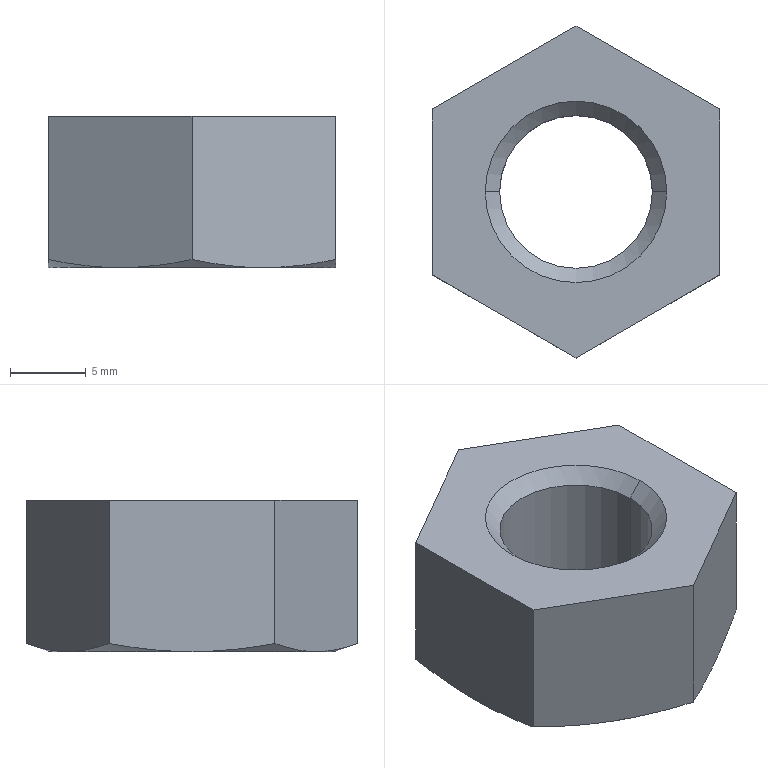Part | SolidWorks | features BaseBody 1 | 1 solid | 20 faces | box 19 x 21.939 x 10 mm | volume 2289 mm3 | cone 10 | plane 8 | cylinder 2 | commonest cylinder face diameters 10.106 x2
STEP:
#1=CARTESIAN_POINT('',(-5.053,0.,0.947));
#2=VERTEX_POINT('',#1);
#3=CARTESIAN_POINT('',(5.053,0.,0.947));
#4=VERTEX_POINT('',#3);
#5=CARTESIAN_POINT('',(0.,0.,0.947));
#6=DIRECTION('',(0.,0.,1.));
#7=DIRECTION('',(1.,0.,0.));
#8=AXIS2_PLACEMENT_3D('',#5,#6,#7);
#9=CIRCLE('',#8,5.053);
#10=EDGE_CURVE('',#2,#4,#9,.T.);
#11=ORIENTED_EDGE('',*,*,#10,.F.);
#12=CARTESIAN_POINT('',(-5.053,0.,9.053));
#13=VERTEX_POINT('',#12);
#14=CARTESIAN_POINT('',(-5.053,0.,0.));
#15=DIRECTION('',(0.,0.,1.));
#16=VECTOR('',#15,1000.);
#17=LINE('',#14,#16);
#18=EDGE_CURVE('',#2,#13,#17,.T.);
#19=ORIENTED_EDGE('',*,*,#18,.T.);
#20=CARTESIAN_POINT('',(5.053,0.,9.053));
#21=VERTEX_POINT('',#20);
#22=CARTESIAN_POINT('',(0.,0.,9.053));
#23=DIRECTION('',(0.,0.,-1.));
#24=DIRECTION('',(1.,0.,0.));
#25=AXIS2_PLACEMENT_3D('',#22,#23,#24);
#26=CIRCLE('',#25,5.053);
#27=EDGE_CURVE('',#21,#13,#26,.T.);
#28=ORIENTED_EDGE('',*,*,#27,.F.);
#29=CARTESIAN_POINT('',(5.053,0.,0.));
#30=DIRECTION('',(0.,0.,1.));
#31=VECTOR('',#30,1000.);
#32=LINE('',#29,#31);
#33=EDGE_CURVE('',#4,#21,#32,.T.);
#34=ORIENTED_EDGE('',*,*,#33,.F.);
#35=EDGE_LOOP('',(#11,#19,#28,#34));
#36=FACE_OUTER_BOUND('',#35,.T.);
#37=CARTESIAN_POINT('',(0.,0.,0.));
#38=DIRECTION('',(0.,0.,1.));
#39=DIRECTION('',(1.,0.,0.));
#40=AXIS2_PLACEMENT_3D('',#37,#38,#39);
#41=CYLINDRICAL_SURFACE('',#40,5.053);
#42=ADVANCED_FACE('',(#36),#41,.F.);
#43=ORIENTED_EDGE('',*,*,#27,.T.);
#44=CARTESIAN_POINT('',(-6.,0.,10.));
#45=VERTEX_POINT('',#44);
#46=CARTESIAN_POINT('',(-6.,0.,10.));
#47=DIRECTION('',(-0.7071,0.,0.7071));
#48=VECTOR('',#47,1000.);
#49=LINE('',#46,#48);
#50=EDGE_CURVE('',#13,#45,#49,.T.);
#51=ORIENTED_EDGE('',*,*,#50,.T.);
#52=CARTESIAN_POINT('',(6.,0.,10.));
#53=VERTEX_POINT('',#52);
#54=CARTESIAN_POINT('',(0.,0.,10.));
#55=DIRECTION('',(0.,0.,-1.));
#56=DIRECTION('',(1.,0.,0.));
#57=AXIS2_PLACEMENT_3D('',#54,#55,#56);
#58=CIRCLE('',#57,6.);
#59=EDGE_CURVE('',#53,#45,#58,.T.);
#60=ORIENTED_EDGE('',*,*,#59,.F.);
#61=CARTESIAN_POINT('',(6.,0.,10.));
#62=DIRECTION('',(0.7071,0.,0.7071));
#63=VECTOR('',#62,1000.);
#64=LINE('',#61,#63);
#65=EDGE_CURVE('',#21,#53,#64,.T.);
#66=ORIENTED_EDGE('',*,*,#65,.F.);
#67=EDGE_LOOP('',(#43,#51,#60,#66));
#68=FACE_OUTER_BOUND('',#67,.T.);
#69=CARTESIAN_POINT('',(0.,0.,10.));
#70=DIRECTION('',(0.,0.,1.));
#71=DIRECTION('',(1.,0.,0.));
#72=AXIS2_PLACEMENT_3D('',#69,#70,#71);
#73=CONICAL_SURFACE('',#72,6.,0.7854);
#74=ADVANCED_FACE('',(#68),#73,.F.);
#75=ORIENTED_EDGE('',*,*,#10,.T.);
#76=CARTESIAN_POINT('',(6.,0.,0.));
#77=VERTEX_POINT('',#76);
#78=CARTESIAN_POINT('',(6.,0.,0.));
#79=DIRECTION('',(0.7071,0.,-0.7071));
#80=VECTOR('',#79,1000.);
#81=LINE('',#78,#80);
#82=EDGE_CURVE('',#4,#77,#81,.T.);
#83=ORIENTED_EDGE('',*,*,#82,.T.);
#84=CARTESIAN_POINT('',(-6.,0.,0.));
#85=VERTEX_POINT('',#84);
#86=CARTESIAN_POINT('',(0.,0.,0.));
#87=DIRECTION('',(0.,0.,1.));
#88=DIRECTION('',(-1.,0.,0.));
#89=AXIS2_PLACEMENT_3D('',#86,#87,#88);
#90=CIRCLE('',#89,6.);
#91=EDGE_CURVE('',#85,#77,#90,.T.);
#92=ORIENTED_EDGE('',*,*,#91,.F.);
#93=CARTESIAN_POINT('',(-6.,0.,0.));
#94=DIRECTION('',(-0.7071,0.,-0.7071));
#95=VECTOR('',#94,1000.);
#96=LINE('',#93,#95);
#97=EDGE_CURVE('',#2,#85,#96,.T.);
#98=ORIENTED_EDGE('',*,*,#97,.F.);
#99=EDGE_LOOP('',(#75,#83,#92,#98));
#100=FACE_OUTER_BOUND('',#99,.T.);
#101=CARTESIAN_POINT('',(0.,0.,0.));
#102=DIRECTION('',(0.,0.,-1.));
#103=DIRECTION('',(-1.,0.,0.));
#104=AXIS2_PLACEMENT_3D('',#101,#102,#103);
#105=CONICAL_SURFACE('',#104,6.,0.7854);
#106=ADVANCED_FACE('',(#100),#105,.F.);
#107=ORIENTED_EDGE('',*,*,#18,.F.);
#108=CARTESIAN_POINT('',(0.,0.,0.947));
#109=DIRECTION('',(0.,0.,1.));
#110=DIRECTION('',(1.,0.,0.));
#111=AXIS2_PLACEMENT_3D('',#108,#109,#110);
#112=CIRCLE('',#111,5.053);
#113=EDGE_CURVE('',#4,#2,#112,.T.);
#114=ORIENTED_EDGE('',*,*,#113,.F.);
#115=ORIENTED_EDGE('',*,*,#33,.T.);
#116=CARTESIAN_POINT('',(0.,0.,9.053));
#117=DIRECTION('',(0.,0.,-1.));
#118=DIRECTION('',(1.,0.,0.));
#119=AXIS2_PLACEMENT_3D('',#116,#117,#118);
#120=CIRCLE('',#119,5.053);
#121=EDGE_CURVE('',#13,#21,#120,.T.);
#122=ORIENTED_EDGE('',*,*,#121,.F.);
#123=EDGE_LOOP('',(#107,#114,#115,#122));
#124=FACE_OUTER_BOUND('',#123,.T.);
#125=CARTESIAN_POINT('',(0.,0.,0.));
#126=DIRECTION('',(0.,0.,1.));
#127=DIRECTION('',(1.,0.,0.));
#128=AXIS2_PLACEMENT_3D('',#125,#126,#127);
#129=CYLINDRICAL_SURFACE('',#128,5.053);
#130=ADVANCED_FACE('',(#124),#129,.F.);
#131=ORIENTED_EDGE('',*,*,#50,.F.);
#132=ORIENTED_EDGE('',*,*,#121,.T.);
#133=ORIENTED_EDGE('',*,*,#65,.T.);
#134=CARTESIAN_POINT('',(0.,0.,10.));
#135=DIRECTION('',(0.,0.,-1.));
#136=DIRECTION('',(1.,0.,0.));
#137=AXIS2_PLACEMENT_3D('',#134,#135,#136);
#138=CIRCLE('',#137,6.);
#139=EDGE_CURVE('',#45,#53,#138,.T.);
#140=ORIENTED_EDGE('',*,*,#139,.F.);
#141=EDGE_LOOP('',(#131,#132,#133,#140));
#142=FACE_OUTER_BOUND('',#141,.T.);
#143=CARTESIAN_POINT('',(0.,0.,10.));
#144=DIRECTION('',(0.,0.,1.));
#145=DIRECTION('',(1.,0.,0.));
#146=AXIS2_PLACEMENT_3D('',#143,#144,#145);
#147=CONICAL_SURFACE('',#146,6.,0.7854);
#148=ADVANCED_FACE('',(#142),#147,.F.);
#149=ORIENTED_EDGE('',*,*,#82,.F.);
#150=ORIENTED_EDGE('',*,*,#113,.T.);
#151=ORIENTED_EDGE('',*,*,#97,.T.);
#152=CARTESIAN_POINT('',(0.,0.,0.));
#153=DIRECTION('',(0.,0.,1.));
#154=DIRECTION('',(-1.,0.,0.));
#155=AXIS2_PLACEMENT_3D('',#152,#153,#154);
#156=CIRCLE('',#155,6.);
#157=EDGE_CURVE('',#77,#85,#156,.T.);
#158=ORIENTED_EDGE('',*,*,#157,.F.);
#159=EDGE_LOOP('',(#149,#150,#151,#158));
#160=FACE_OUTER_BOUND('',#159,.T.);
#161=CARTESIAN_POINT('',(0.,0.,0.));
#162=DIRECTION('',(0.,0.,-1.));
#163=DIRECTION('',(-1.,0.,0.));
#164=AXIS2_PLACEMENT_3D('',#161,#162,#163);
#165=CONICAL_SURFACE('',#164,6.,0.7854);
#166=ADVANCED_FACE('',(#160),#165,.F.);
#167=ORIENTED_EDGE('',*,*,#59,.T.);
#168=ORIENTED_EDGE('',*,*,#139,.T.);
#169=EDGE_LOOP('',(#167,#168));
#170=FACE_BOUND('',#169,.T.);
#171=CARTESIAN_POINT('',(9.5,-5.485,10.));
#172=VERTEX_POINT('',#171);
#173=CARTESIAN_POINT('',(9.5,5.485,10.));
#174=VERTEX_POINT('',#173);
#175=CARTESIAN_POINT('',(9.5,0.,10.));
#176=DIRECTION('',(0.,1.,0.));
#177=VECTOR('',#176,1000.);
#178=LINE('',#175,#177);
#179=EDGE_CURVE('',#172,#174,#178,.T.);
#180=ORIENTED_EDGE('',*,*,#179,.T.);
#181=CARTESIAN_POINT('',(0.,10.97,10.));
#182=VERTEX_POINT('',#181);
#183=CARTESIAN_POINT('',(9.5,5.485,10.));
#184=DIRECTION('',(-0.866,0.5,0.));
#185=VECTOR('',#184,1000.);
#186=LINE('',#183,#185);
#187=EDGE_CURVE('',#174,#182,#186,.T.);
#188=ORIENTED_EDGE('',*,*,#187,.T.);
#189=CARTESIAN_POINT('',(-9.5,5.485,10.));
#190=VERTEX_POINT('',#189);
#191=CARTESIAN_POINT('',(0.,10.97,10.));
#192=DIRECTION('',(-0.866,-0.5,0.));
#193=VECTOR('',#192,1000.);
#194=LINE('',#191,#193);
#195=EDGE_CURVE('',#182,#190,#194,.T.);
#196=ORIENTED_EDGE('',*,*,#195,.T.);
#197=CARTESIAN_POINT('',(-9.5,-5.485,10.));
#198=VERTEX_POINT('',#197);
#199=CARTESIAN_POINT('',(-9.5,0.,10.));
#200=DIRECTION('',(0.,-1.,0.));
#201=VECTOR('',#200,1000.);
#202=LINE('',#199,#201);
#203=EDGE_CURVE('',#190,#198,#202,.T.);
#204=ORIENTED_EDGE('',*,*,#203,.T.);
#205=CARTESIAN_POINT('',(0.,-10.97,10.));
#206=VERTEX_POINT('',#205);
#207=CARTESIAN_POINT('',(-9.5,-5.485,10.));
#208=DIRECTION('',(0.866,-0.5,0.));
#209=VECTOR('',#208,1000.);
#210=LINE('',#207,#209);
#211=EDGE_CURVE('',#198,#206,#210,.T.);
#212=ORIENTED_EDGE('',*,*,#211,.T.);
#213=CARTESIAN_POINT('',(0.,-10.97,10.));
#214=DIRECTION('',(0.866,0.5,0.));
#215=VECTOR('',#214,1000.);
#216=LINE('',#213,#215);
#217=EDGE_CURVE('',#206,#172,#216,.T.);
#218=ORIENTED_EDGE('',*,*,#217,.T.);
#219=EDGE_LOOP('',(#180,#188,#196,#204,#212,#218));
#220=FACE_OUTER_BOUND('',#219,.T.);
#221=CARTESIAN_POINT('',(0.,0.,10.));
#222=DIRECTION('',(0.,0.,1.));
#223=DIRECTION('',(1.,0.,0.));
#224=AXIS2_PLACEMENT_3D('',#221,#222,#223);
#225=PLANE('',#224);
#226=ADVANCED_FACE('',(#170,#220),#225,.T.);
#227=ORIENTED_EDGE('',*,*,#91,.T.);
#228=ORIENTED_EDGE('',*,*,#157,.T.);
#229=EDGE_LOOP('',(#227,#228));
#230=FACE_BOUND('',#229,.T.);
#231=CARTESIAN_POINT('',(-4.75,-8.227,0.));
#232=VERTEX_POINT('',#231);
#233=CARTESIAN_POINT('',(4.75,-8.227,0.));
#234=VERTEX_POINT('',#233);
#235=CARTESIAN_POINT('',(0.,0.,0.));
#236=DIRECTION('',(0.,0.,1.));
#237=DIRECTION('',(1.,0.,0.));
#238=AXIS2_PLACEMENT_3D('',#235,#236,#237);
#239=CIRCLE('',#238,9.5);
#240=EDGE_CURVE('',#232,#234,#239,.T.);
#241=ORIENTED_EDGE('',*,*,#240,.F.);
#242=CARTESIAN_POINT('',(-9.5,0.,0.));
#243=VERTEX_POINT('',#242);
#244=CARTESIAN_POINT('',(0.,0.,0.));
#245=DIRECTION('',(0.,0.,1.));
#246=DIRECTION('',(1.,0.,0.));
#247=AXIS2_PLACEMENT_3D('',#244,#245,#246);
#248=CIRCLE('',#247,9.5);
#249=EDGE_CURVE('',#243,#232,#248,.T.);
#250=ORIENTED_EDGE('',*,*,#249,.F.);
#251=CARTESIAN_POINT('',(-4.75,8.227,0.));
#252=VERTEX_POINT('',#251);
#253=CARTESIAN_POINT('',(0.,0.,0.));
#254=DIRECTION('',(0.,0.,1.));
#255=DIRECTION('',(1.,0.,0.));
#256=AXIS2_PLACEMENT_3D('',#253,#254,#255);
#257=CIRCLE('',#256,9.5);
#258=EDGE_CURVE('',#252,#243,#257,.T.);
#259=ORIENTED_EDGE('',*,*,#258,.F.);
#260=CARTESIAN_POINT('',(4.75,8.227,0.));
#261=VERTEX_POINT('',#260);
#262=CARTESIAN_POINT('',(0.,0.,0.));
#263=DIRECTION('',(0.,0.,1.));
#264=DIRECTION('',(1.,0.,0.));
#265=AXIS2_PLACEMENT_3D('',#262,#263,#264);
#266=CIRCLE('',#265,9.5);
#267=EDGE_CURVE('',#261,#252,#266,.T.);
#268=ORIENTED_EDGE('',*,*,#267,.F.);
#269=CARTESIAN_POINT('',(9.5,0.,0.));
#270=VERTEX_POINT('',#269);
#271=CARTESIAN_POINT('',(0.,0.,0.));
#272=DIRECTION('',(0.,0.,1.));
#273=DIRECTION('',(1.,0.,0.));
#274=AXIS2_PLACEMENT_3D('',#271,#272,#273);
#275=CIRCLE('',#274,9.5);
#276=EDGE_CURVE('',#270,#261,#275,.T.);
#277=ORIENTED_EDGE('',*,*,#276,.F.);
#278=CARTESIAN_POINT('',(0.,0.,0.));
#279=DIRECTION('',(0.,0.,1.));
#280=DIRECTION('',(1.,0.,0.));
#281=AXIS2_PLACEMENT_3D('',#278,#279,#280);
#282=CIRCLE('',#281,9.5);
#283=EDGE_CURVE('',#234,#270,#282,.T.);
#284=ORIENTED_EDGE('',*,*,#283,.F.);
#285=EDGE_LOOP('',(#241,#250,#259,#268,#277,#284));
#286=FACE_OUTER_BOUND('',#285,.T.);
#287=CARTESIAN_POINT('',(0.,0.,0.));
#288=DIRECTION('',(0.,0.,1.));
#289=DIRECTION('',(1.,0.,0.));
#290=AXIS2_PLACEMENT_3D('',#287,#288,#289);
#291=PLANE('',#290);
#292=ADVANCED_FACE('',(#230,#286),#291,.F.);
#293=CARTESIAN_POINT('',(9.5,5.485,0.5349));
#294=VERTEX_POINT('',#293);
#295=CARTESIAN_POINT('',(4.75,8.227,0.));
#296=CARTESIAN_POINT('',(5.549,7.766,0.));
#297=CARTESIAN_POINT('',(6.344,7.307,0.0498));
#298=CARTESIAN_POINT('',(7.927,6.393,0.235));
#299=CARTESIAN_POINT('',(8.715,5.938,0.3699));
#300=CARTESIAN_POINT('',(9.5,5.485,0.5349));
#301=B_SPLINE_CURVE_WITH_KNOTS('',3,(#295,#296,#297,#298,#299,#300),.UNSPECIFIED.,.F.,.F.,(4,2,4),(0.,0.002755,0.005511),.UNSPECIFIED.);
#302=EDGE_CURVE('',#261,#294,#301,.T.);
#303=ORIENTED_EDGE('',*,*,#302,.F.);
#304=CARTESIAN_POINT('',(0.,10.97,0.5349));
#305=VERTEX_POINT('',#304);
#306=CARTESIAN_POINT('',(0.,10.97,0.5349));
#307=CARTESIAN_POINT('',(0.7853,10.516,0.3699));
#308=CARTESIAN_POINT('',(1.573,10.061,0.235));
#309=CARTESIAN_POINT('',(3.156,9.148,0.0498));
#310=CARTESIAN_POINT('',(3.951,8.689,0.));
#311=CARTESIAN_POINT('',(4.75,8.227,0.));
#312=B_SPLINE_CURVE_WITH_KNOTS('',3,(#306,#307,#308,#309,#310,#311),.UNSPECIFIED.,.F.,.F.,(4,2,4),(0.,0.002755,0.005511),.UNSPECIFIED.);
#313=EDGE_CURVE('',#305,#261,#312,.T.);
#314=ORIENTED_EDGE('',*,*,#313,.F.);
#315=CARTESIAN_POINT('',(0.,10.97,10.));
#316=DIRECTION('',(0.,0.,-1.));
#317=VECTOR('',#316,1000.);
#318=LINE('',#315,#317);
#319=EDGE_CURVE('',#182,#305,#318,.T.);
#320=ORIENTED_EDGE('',*,*,#319,.F.);
#321=ORIENTED_EDGE('',*,*,#187,.F.);
#322=CARTESIAN_POINT('',(9.5,5.485,10.));
#323=DIRECTION('',(0.,0.,1.));
#324=VECTOR('',#323,1000.);
#325=LINE('',#322,#324);
#326=EDGE_CURVE('',#294,#174,#325,.T.);
#327=ORIENTED_EDGE('',*,*,#326,.F.);
#328=EDGE_LOOP('',(#303,#314,#320,#321,#327));
#329=FACE_OUTER_BOUND('',#328,.T.);
#330=CARTESIAN_POINT('',(9.5,5.485,10.));
#331=DIRECTION('',(-0.5,-0.866,0.));
#332=DIRECTION('',(0.866,-0.5,0.));
#333=AXIS2_PLACEMENT_3D('',#330,#331,#332);
#334=PLANE('',#333);
#335=ADVANCED_FACE('',(#329),#334,.F.);
#336=CARTESIAN_POINT('',(9.5,-5.485,0.5349));
#337=VERTEX_POINT('',#336);
#338=CARTESIAN_POINT('',(9.5,0.,0.));
#339=CARTESIAN_POINT('',(9.5,-0.9228,0.));
#340=CARTESIAN_POINT('',(9.5,-1.841,0.0498));
#341=CARTESIAN_POINT('',(9.5,-3.668,0.235));
#342=CARTESIAN_POINT('',(9.5,-4.578,0.3699));
#343=CARTESIAN_POINT('',(9.5,-5.485,0.5349));
#344=B_SPLINE_CURVE_WITH_KNOTS('',3,(#338,#339,#340,#341,#342,#343),.UNSPECIFIED.,.F.,.F.,(4,2,4),(0.,0.002755,0.005511),.UNSPECIFIED.);
#345=EDGE_CURVE('',#270,#337,#344,.T.);
#346=ORIENTED_EDGE('',*,*,#345,.F.);
#347=CARTESIAN_POINT('',(9.5,5.485,0.5349));
#348=CARTESIAN_POINT('',(9.5,4.578,0.3699));
#349=CARTESIAN_POINT('',(9.5,3.668,0.235));
#350=CARTESIAN_POINT('',(9.5,1.841,0.0498));
#351=CARTESIAN_POINT('',(9.5,0.9228,0.));
#352=CARTESIAN_POINT('',(9.5,0.,0.));
#353=B_SPLINE_CURVE_WITH_KNOTS('',3,(#347,#348,#349,#350,#351,#352),.UNSPECIFIED.,.F.,.F.,(4,2,4),(0.,0.002755,0.005511),.UNSPECIFIED.);
#354=EDGE_CURVE('',#294,#270,#353,.T.);
#355=ORIENTED_EDGE('',*,*,#354,.F.);
#356=ORIENTED_EDGE('',*,*,#326,.T.);
#357=ORIENTED_EDGE('',*,*,#179,.F.);
#358=CARTESIAN_POINT('',(9.5,-5.485,10.));
#359=DIRECTION('',(0.,0.,1.));
#360=VECTOR('',#359,1000.);
#361=LINE('',#358,#360);
#362=EDGE_CURVE('',#337,#172,#361,.T.);
#363=ORIENTED_EDGE('',*,*,#362,.F.);
#364=EDGE_LOOP('',(#346,#355,#356,#357,#363));
#365=FACE_OUTER_BOUND('',#364,.T.);
#366=CARTESIAN_POINT('',(9.5,-5.485,10.));
#367=DIRECTION('',(-1.,0.,0.));
#368=DIRECTION('',(0.,0.,1.));
#369=AXIS2_PLACEMENT_3D('',#366,#367,#368);
#370=PLANE('',#369);
#371=ADVANCED_FACE('',(#365),#370,.F.);
#372=CARTESIAN_POINT('',(0.,-10.97,0.5349));
#373=VERTEX_POINT('',#372);
#374=CARTESIAN_POINT('',(4.75,-8.227,0.));
#375=CARTESIAN_POINT('',(3.951,-8.689,0.));
#376=CARTESIAN_POINT('',(3.156,-9.148,0.0498));
#377=CARTESIAN_POINT('',(1.573,-10.061,0.235));
#378=CARTESIAN_POINT('',(0.7853,-10.516,0.3699));
#379=CARTESIAN_POINT('',(0.,-10.97,0.5349));
#380=B_SPLINE_CURVE_WITH_KNOTS('',3,(#374,#375,#376,#377,#378,#379),.UNSPECIFIED.,.F.,.F.,(4,2,4),(0.,0.002755,0.005511),.UNSPECIFIED.);
#381=EDGE_CURVE('',#234,#373,#380,.T.);
#382=ORIENTED_EDGE('',*,*,#381,.F.);
#383=CARTESIAN_POINT('',(9.5,-5.485,0.5349));
#384=CARTESIAN_POINT('',(8.715,-5.938,0.3699));
#385=CARTESIAN_POINT('',(7.927,-6.393,0.235));
#386=CARTESIAN_POINT('',(6.344,-7.307,0.0498));
#387=CARTESIAN_POINT('',(5.549,-7.766,0.));
#388=CARTESIAN_POINT('',(4.75,-8.227,0.));
#389=B_SPLINE_CURVE_WITH_KNOTS('',3,(#383,#384,#385,#386,#387,#388),.UNSPECIFIED.,.F.,.F.,(4,2,4),(0.,0.002755,0.005511),.UNSPECIFIED.);
#390=EDGE_CURVE('',#337,#234,#389,.T.);
#391=ORIENTED_EDGE('',*,*,#390,.F.);
#392=ORIENTED_EDGE('',*,*,#362,.T.);
#393=ORIENTED_EDGE('',*,*,#217,.F.);
#394=CARTESIAN_POINT('',(0.,-10.97,10.));
#395=DIRECTION('',(0.,0.,1.));
#396=VECTOR('',#395,1000.);
#397=LINE('',#394,#396);
#398=EDGE_CURVE('',#373,#206,#397,.T.);
#399=ORIENTED_EDGE('',*,*,#398,.F.);
#400=EDGE_LOOP('',(#382,#391,#392,#393,#399));
#401=FACE_OUTER_BOUND('',#400,.T.);
#402=CARTESIAN_POINT('',(0.,-10.97,10.));
#403=DIRECTION('',(-0.5,0.866,0.));
#404=DIRECTION('',(-0.866,-0.5,0.));
#405=AXIS2_PLACEMENT_3D('',#402,#403,#404);
#406=PLANE('',#405);
#407=ADVANCED_FACE('',(#401),#406,.F.);
#408=CARTESIAN_POINT('',(-9.5,-5.485,0.5349));
#409=VERTEX_POINT('',#408);
#410=CARTESIAN_POINT('',(-4.75,-8.227,0.));
#411=CARTESIAN_POINT('',(-5.549,-7.766,0.));
#412=CARTESIAN_POINT('',(-6.344,-7.307,0.0498));
#413=CARTESIAN_POINT('',(-7.927,-6.393,0.235));
#414=CARTESIAN_POINT('',(-8.715,-5.938,0.3699));
#415=CARTESIAN_POINT('',(-9.5,-5.485,0.5349));
#416=B_SPLINE_CURVE_WITH_KNOTS('',3,(#410,#411,#412,#413,#414,#415),.UNSPECIFIED.,.F.,.F.,(4,2,4),(0.,0.002755,0.005511),.UNSPECIFIED.);
#417=EDGE_CURVE('',#232,#409,#416,.T.);
#418=ORIENTED_EDGE('',*,*,#417,.F.);
#419=CARTESIAN_POINT('',(0.,-10.97,0.5349));
#420=CARTESIAN_POINT('',(-0.7853,-10.516,0.3699));
#421=CARTESIAN_POINT('',(-1.573,-10.061,0.235));
#422=CARTESIAN_POINT('',(-3.156,-9.148,0.0498));
#423=CARTESIAN_POINT('',(-3.951,-8.689,0.));
#424=CARTESIAN_POINT('',(-4.75,-8.227,0.));
#425=B_SPLINE_CURVE_WITH_KNOTS('',3,(#419,#420,#421,#422,#423,#424),.UNSPECIFIED.,.F.,.F.,(4,2,4),(0.,0.002755,0.005511),.UNSPECIFIED.);
#426=EDGE_CURVE('',#373,#232,#425,.T.);
#427=ORIENTED_EDGE('',*,*,#426,.F.);
#428=ORIENTED_EDGE('',*,*,#398,.T.);
#429=ORIENTED_EDGE('',*,*,#211,.F.);
#430=CARTESIAN_POINT('',(-9.5,-5.485,10.));
#431=DIRECTION('',(0.,0.,1.));
#432=VECTOR('',#431,1000.);
#433=LINE('',#430,#432);
#434=EDGE_CURVE('',#409,#198,#433,.T.);
#435=ORIENTED_EDGE('',*,*,#434,.F.);
#436=EDGE_LOOP('',(#418,#427,#428,#429,#435));
#437=FACE_OUTER_BOUND('',#436,.T.);
#438=CARTESIAN_POINT('',(-9.5,-5.485,10.));
#439=DIRECTION('',(0.5,0.866,0.));
#440=DIRECTION('',(-0.866,0.5,0.));
#441=AXIS2_PLACEMENT_3D('',#438,#439,#440);
#442=PLANE('',#441);
#443=ADVANCED_FACE('',(#437),#442,.F.);
#444=CARTESIAN_POINT('',(-9.5,5.485,0.5349));
#445=VERTEX_POINT('',#444);
#446=CARTESIAN_POINT('',(-9.5,0.,0.));
#447=CARTESIAN_POINT('',(-9.5,0.9228,0.));
#448=CARTESIAN_POINT('',(-9.5,1.841,0.0498));
#449=CARTESIAN_POINT('',(-9.5,3.668,0.235));
#450=CARTESIAN_POINT('',(-9.5,4.578,0.3699));
#451=CARTESIAN_POINT('',(-9.5,5.485,0.5349));
#452=B_SPLINE_CURVE_WITH_KNOTS('',3,(#446,#447,#448,#449,#450,#451),.UNSPECIFIED.,.F.,.F.,(4,2,4),(0.,0.002755,0.005511),.UNSPECIFIED.);
#453=EDGE_CURVE('',#243,#445,#452,.T.);
#454=ORIENTED_EDGE('',*,*,#453,.F.);
#455=CARTESIAN_POINT('',(-9.5,-5.485,0.5349));
#456=CARTESIAN_POINT('',(-9.5,-4.578,0.3699));
#457=CARTESIAN_POINT('',(-9.5,-3.668,0.235));
#458=CARTESIAN_POINT('',(-9.5,-1.841,0.0498));
#459=CARTESIAN_POINT('',(-9.5,-0.9228,0.));
#460=CARTESIAN_POINT('',(-9.5,0.,0.));
#461=B_SPLINE_CURVE_WITH_KNOTS('',3,(#455,#456,#457,#458,#459,#460),.UNSPECIFIED.,.F.,.F.,(4,2,4),(0.,0.002755,0.005511),.UNSPECIFIED.);
#462=EDGE_CURVE('',#409,#243,#461,.T.);
#463=ORIENTED_EDGE('',*,*,#462,.F.);
#464=ORIENTED_EDGE('',*,*,#434,.T.);
#465=ORIENTED_EDGE('',*,*,#203,.F.);
#466=CARTESIAN_POINT('',(-9.5,5.485,10.));
#467=DIRECTION('',(0.,0.,1.));
#468=VECTOR('',#467,1000.);
#469=LINE('',#466,#468);
#470=EDGE_CURVE('',#445,#190,#469,.T.);
#471=ORIENTED_EDGE('',*,*,#470,.F.);
#472=EDGE_LOOP('',(#454,#463,#464,#465,#471));
#473=FACE_OUTER_BOUND('',#472,.T.);
#474=CARTESIAN_POINT('',(-9.5,5.485,10.));
#475=DIRECTION('',(1.,0.,0.));
#476=DIRECTION('',(0.,0.,-1.));
#477=AXIS2_PLACEMENT_3D('',#474,#475,#476);
#478=PLANE('',#477);
#479=ADVANCED_FACE('',(#473),#478,.F.);
#480=CARTESIAN_POINT('',(-4.75,8.227,0.));
#481=CARTESIAN_POINT('',(-3.951,8.689,0.));
#482=CARTESIAN_POINT('',(-3.156,9.148,0.0498));
#483=CARTESIAN_POINT('',(-1.573,10.061,0.235));
#484=CARTESIAN_POINT('',(-0.7853,10.516,0.3699));
#485=CARTESIAN_POINT('',(0.,10.97,0.5349));
#486=B_SPLINE_CURVE_WITH_KNOTS('',3,(#480,#481,#482,#483,#484,#485),.UNSPECIFIED.,.F.,.F.,(4,2,4),(0.,0.002755,0.005511),.UNSPECIFIED.);
#487=EDGE_CURVE('',#252,#305,#486,.T.);
#488=ORIENTED_EDGE('',*,*,#487,.F.);
#489=CARTESIAN_POINT('',(-9.5,5.485,0.5349));
#490=CARTESIAN_POINT('',(-8.715,5.938,0.3699));
#491=CARTESIAN_POINT('',(-7.927,6.393,0.235));
#492=CARTESIAN_POINT('',(-6.344,7.307,0.0498));
#493=CARTESIAN_POINT('',(-5.549,7.766,0.));
#494=CARTESIAN_POINT('',(-4.75,8.227,0.));
#495=B_SPLINE_CURVE_WITH_KNOTS('',3,(#489,#490,#491,#492,#493,#494),.UNSPECIFIED.,.F.,.F.,(4,2,4),(0.,0.002755,0.005511),.UNSPECIFIED.);
#496=EDGE_CURVE('',#445,#252,#495,.T.);
#497=ORIENTED_EDGE('',*,*,#496,.F.);
#498=ORIENTED_EDGE('',*,*,#470,.T.);
#499=ORIENTED_EDGE('',*,*,#195,.F.);
#500=ORIENTED_EDGE('',*,*,#319,.T.);
#501=EDGE_LOOP('',(#488,#497,#498,#499,#500));
#502=FACE_OUTER_BOUND('',#501,.T.);
#503=CARTESIAN_POINT('',(0.,10.97,10.));
#504=DIRECTION('',(0.5,-0.866,0.));
#505=DIRECTION('',(0.866,0.5,0.));
#506=AXIS2_PLACEMENT_3D('',#503,#504,#505);
#507=PLANE('',#506);
#508=ADVANCED_FACE('',(#502),#507,.F.);
#509=ORIENTED_EDGE('',*,*,#345,.T.);
#510=ORIENTED_EDGE('',*,*,#390,.T.);
#511=ORIENTED_EDGE('',*,*,#283,.T.);
#512=EDGE_LOOP('',(#509,#510,#511));
#513=FACE_OUTER_BOUND('',#512,.T.);
#514=CARTESIAN_POINT('',(0.,0.,0.5381));
#515=DIRECTION('',(0.,0.,1.));
#516=DIRECTION('',(1.,0.,0.));
#517=AXIS2_PLACEMENT_3D('',#514,#515,#516);
#518=CONICAL_SURFACE('',#517,10.978,1.222);
#519=ADVANCED_FACE('',(#513),#518,.T.);
#520=ORIENTED_EDGE('',*,*,#381,.T.);
#521=ORIENTED_EDGE('',*,*,#426,.T.);
#522=ORIENTED_EDGE('',*,*,#240,.T.);
#523=EDGE_LOOP('',(#520,#521,#522));
#524=FACE_OUTER_BOUND('',#523,.T.);
#525=CARTESIAN_POINT('',(0.,0.,0.5381));
#526=DIRECTION('',(0.,0.,1.));
#527=DIRECTION('',(1.,0.,0.));
#528=AXIS2_PLACEMENT_3D('',#525,#526,#527);
#529=CONICAL_SURFACE('',#528,10.978,1.222);
#530=ADVANCED_FACE('',(#524),#529,.T.);
#531=ORIENTED_EDGE('',*,*,#417,.T.);
#532=ORIENTED_EDGE('',*,*,#462,.T.);
#533=ORIENTED_EDGE('',*,*,#249,.T.);
#534=EDGE_LOOP('',(#531,#532,#533));
#535=FACE_OUTER_BOUND('',#534,.T.);
#536=CARTESIAN_POINT('',(0.,0.,0.5381));
#537=DIRECTION('',(0.,0.,1.));
#538=DIRECTION('',(1.,0.,0.));
#539=AXIS2_PLACEMENT_3D('',#536,#537,#538);
#540=CONICAL_SURFACE('',#539,10.978,1.222);
#541=ADVANCED_FACE('',(#535),#540,.T.);
#542=ORIENTED_EDGE('',*,*,#453,.T.);
#543=ORIENTED_EDGE('',*,*,#496,.T.);
#544=ORIENTED_EDGE('',*,*,#258,.T.);
#545=EDGE_LOOP('',(#542,#543,#544));
#546=FACE_OUTER_BOUND('',#545,.T.);
#547=CARTESIAN_POINT('',(0.,0.,0.5381));
#548=DIRECTION('',(0.,0.,1.));
#549=DIRECTION('',(1.,0.,0.));
#550=AXIS2_PLACEMENT_3D('',#547,#548,#549);
#551=CONICAL_SURFACE('',#550,10.978,1.222);
#552=ADVANCED_FACE('',(#546),#551,.T.);
#553=ORIENTED_EDGE('',*,*,#313,.T.);
#554=ORIENTED_EDGE('',*,*,#267,.T.);
#555=ORIENTED_EDGE('',*,*,#487,.T.);
#556=EDGE_LOOP('',(#553,#554,#555));
#557=FACE_OUTER_BOUND('',#556,.T.);
#558=CARTESIAN_POINT('',(0.,0.,0.5381));
#559=DIRECTION('',(0.,0.,1.));
#560=DIRECTION('',(1.,0.,0.));
#561=AXIS2_PLACEMENT_3D('',#558,#559,#560);
#562=CONICAL_SURFACE('',#561,10.978,1.222);
#563=ADVANCED_FACE('',(#557),#562,.T.);
#564=ORIENTED_EDGE('',*,*,#302,.T.);
#565=ORIENTED_EDGE('',*,*,#354,.T.);
#566=ORIENTED_EDGE('',*,*,#276,.T.);
#567=EDGE_LOOP('',(#564,#565,#566));
#568=FACE_OUTER_BOUND('',#567,.T.);
#569=CARTESIAN_POINT('',(0.,0.,0.5381));
#570=DIRECTION('',(0.,0.,1.));
#571=DIRECTION('',(1.,0.,0.));
#572=AXIS2_PLACEMENT_3D('',#569,#570,#571);
#573=CONICAL_SURFACE('',#572,10.978,1.222);
#574=ADVANCED_FACE('',(#568),#573,.T.);
#575=CLOSED_SHELL('',(#42,#74,#106,#130,#148,#166,#226,#292,#335,#371,#407,#443,#479,#508,#519,#530,#541,#552,#563,#574));
#576=MANIFOLD_SOLID_BREP('',#575);
#577=CARTESIAN_POINT('',(0.,0.,0.));
#578=DIRECTION('',(0.,0.,1.));
#579=DIRECTION('',(1.,0.,0.));
#580=AXIS2_PLACEMENT_3D('',#577,#578,#579);
#581=(LENGTH_UNIT()NAMED_UNIT(*)SI_UNIT(.MILLI.,.METRE.));
#582=UNCERTAINTY_MEASURE_WITH_UNIT(LENGTH_MEASURE(0.00001),#581,'','');
#583=(NAMED_UNIT(*)PLANE_ANGLE_UNIT()SI_UNIT($,.RADIAN.));
#584=(NAMED_UNIT(*)SI_UNIT($,.STERADIAN.)SOLID_ANGLE_UNIT());
#585=(GEOMETRIC_REPRESENTATION_CONTEXT(3)GLOBAL_UNCERTAINTY_ASSIGNED_CONTEXT((#582))GLOBAL_UNIT_ASSIGNED_CONTEXT((#581,#583,#584))REPRESENTATION_CONTEXT('',''));
#586=ADVANCED_BREP_SHAPE_REPRESENTATION('',(#576,#580),#585);